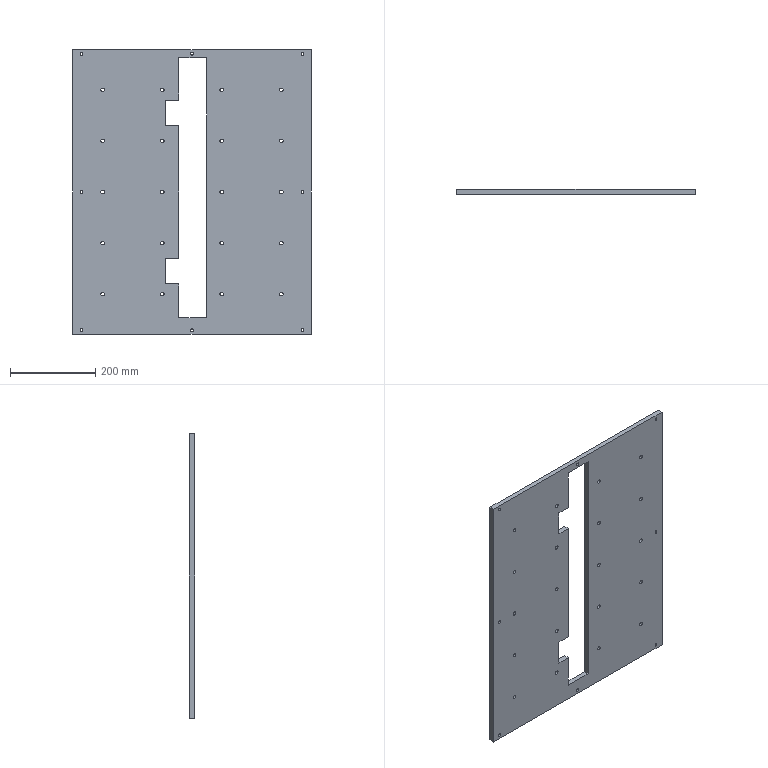Part | SolidWorks | features MirrorPattern 3, Cut 2, Extrusion 1, HoleWzd 1, ICE 1 | 1 solid | 90 faces | box 560 x 12 x 670 mm | volume 3956531 mm3 | cylinder 56 | plane 18 | cone 16 | commonest cylinder face diameters 8.5 x40 6.6 x16